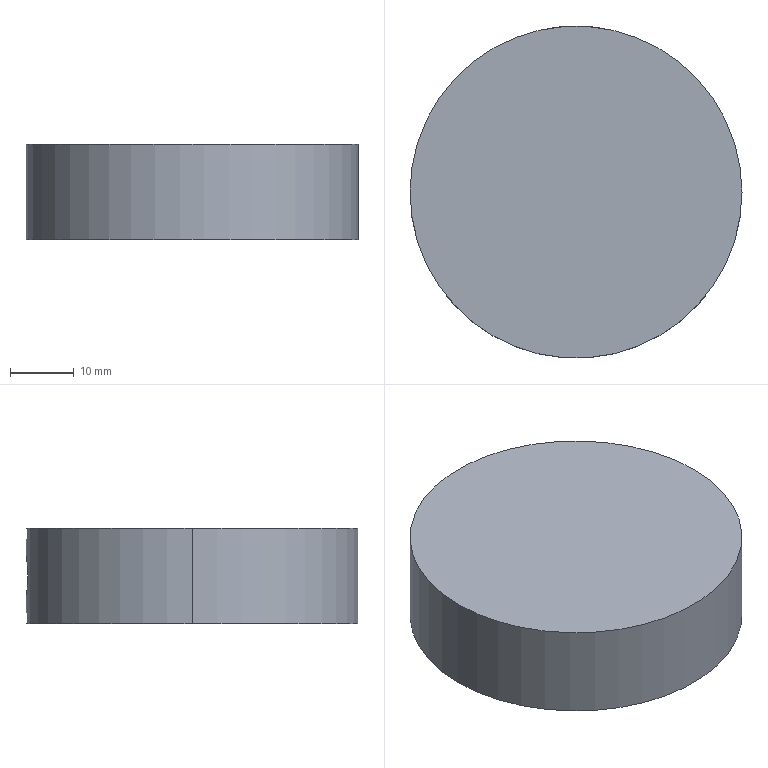Part | SolidWorks | features Extrusion 1, RevCut 1 | 1 solid | 8 faces | box 52 x 52 x 15 mm | volume 31469 mm3 | cylinder 4 | cone 2 | plane 2 | commonest cylinder face diameters 6.8 x2 52 x2
STEP:
#1=CARTESIAN_POINT('',(-106.5,85.3,0.));
#2=VERTEX_POINT('',#1);
#3=CARTESIAN_POINT('',(-109.9,87.263,0.));
#4=VERTEX_POINT('',#3);
#5=CARTESIAN_POINT('',(-106.5,85.3,0.));
#6=DIRECTION('',(-0.866,0.5,0.));
#7=VECTOR('',#6,1000.);
#8=LINE('',#5,#7);
#9=EDGE_CURVE('',#2,#4,#8,.T.);
#10=ORIENTED_EDGE('',*,*,#9,.F.);
#11=CARTESIAN_POINT('',(-103.1,87.263,0.));
#12=VERTEX_POINT('',#11);
#13=CARTESIAN_POINT('',(-106.5,85.3,0.));
#14=DIRECTION('',(0.866,0.5,0.));
#15=VECTOR('',#14,1000.);
#16=LINE('',#13,#15);
#17=EDGE_CURVE('',#2,#12,#16,.T.);
#18=ORIENTED_EDGE('',*,*,#17,.T.);
#19=CARTESIAN_POINT('',(-106.5,87.263,0.));
#20=DIRECTION('',(0.,-1.,0.));
#21=DIRECTION('',(1.,0.,0.));
#22=AXIS2_PLACEMENT_3D('',#19,#20,#21);
#23=CIRCLE('',#22,3.4);
#24=EDGE_CURVE('',#4,#12,#23,.T.);
#25=ORIENTED_EDGE('',*,*,#24,.F.);
#26=EDGE_LOOP('',(#10,#18,#25));
#27=FACE_OUTER_BOUND('',#26,.T.);
#28=CARTESIAN_POINT('',(-106.5,1085.3,0.));
#29=DIRECTION('',(0.,1.,0.));
#30=DIRECTION('',(-1.,0.,0.));
#31=AXIS2_PLACEMENT_3D('',#28,#29,#30);
#32=CONICAL_SURFACE('',#31,1732.051,1.047);
#33=ADVANCED_FACE('',(#27),#32,.F.);
#34=CARTESIAN_POINT('',(-109.9,97.077,0.));
#35=VERTEX_POINT('',#34);
#36=CARTESIAN_POINT('',(-103.1,97.077,0.));
#37=VERTEX_POINT('',#36);
#38=CARTESIAN_POINT('',(-109.9,97.077,0.));
#39=CARTESIAN_POINT('',(-109.9,97.077,-0.2248));
#40=CARTESIAN_POINT('',(-109.878,97.08,-0.4458));
#41=CARTESIAN_POINT('',(-109.791,97.091,-0.8807));
#42=CARTESIAN_POINT('',(-109.726,97.099,-1.097));
#43=CARTESIAN_POINT('',(-109.555,97.12,-1.508));
#44=CARTESIAN_POINT('',(-109.451,97.132,-1.703));
#45=CARTESIAN_POINT('',(-109.204,97.159,-2.073));
#46=CARTESIAN_POINT('',(-109.061,97.174,-2.248));
#47=CARTESIAN_POINT('',(-108.748,97.203,-2.561));
#48=CARTESIAN_POINT('',(-108.577,97.218,-2.701));
#49=CARTESIAN_POINT('',(-108.205,97.245,-2.95));
#50=CARTESIAN_POINT('',(-108.008,97.257,-3.056));
#51=CARTESIAN_POINT('',(-107.599,97.278,-3.225));
#52=CARTESIAN_POINT('',(-107.384,97.286,-3.291));
#53=CARTESIAN_POINT('',(-106.945,97.297,-3.378));
#54=CARTESIAN_POINT('',(-106.722,97.3,-3.4));
#55=CARTESIAN_POINT('',(-106.273,97.3,-3.4));
#56=CARTESIAN_POINT('',(-106.052,97.297,-3.378));
#57=CARTESIAN_POINT('',(-105.617,97.286,-3.291));
#58=CARTESIAN_POINT('',(-105.401,97.278,-3.225));
#59=CARTESIAN_POINT('',(-104.989,97.257,-3.054));
#60=CARTESIAN_POINT('',(-104.794,97.245,-2.95));
#61=CARTESIAN_POINT('',(-104.425,97.218,-2.703));
#62=CARTESIAN_POINT('',(-104.251,97.203,-2.559));
#63=CARTESIAN_POINT('',(-103.938,97.174,-2.246));
#64=CARTESIAN_POINT('',(-103.797,97.159,-2.075));
#65=CARTESIAN_POINT('',(-103.549,97.132,-1.703));
#66=CARTESIAN_POINT('',(-103.443,97.12,-1.505));
#67=CARTESIAN_POINT('',(-103.274,97.099,-1.096));
#68=CARTESIAN_POINT('',(-103.209,97.091,-0.8817));
#69=CARTESIAN_POINT('',(-103.122,97.08,-0.4427));
#70=CARTESIAN_POINT('',(-103.1,97.077,-0.222));
#71=CARTESIAN_POINT('',(-103.1,97.077,0.));
#72=B_SPLINE_CURVE_WITH_KNOTS('',3,(#38,#39,#40,#41,#42,#43,#44,#45,#46,#47,#48,#49,#50,#51,#52,#53,#54,#55,#56,#57,#58,#59,#60,#61,#62,#63,#64,#65,#66,#67,#68,#69,#70,#71),.UNSPECIFIED.,.F.,.F.,(4,2,2,2,2,2,2,2,2,2,2,2,2,2,2,2,4),(0.01596,0.01663,0.01729,0.01796,0.01862,0.01929,0.01995,0.02062,0.02128,0.02195,0.02261,0.02328,0.02394,0.02461,0.02527,0.02594,0.0266),.UNSPECIFIED.);
#73=EDGE_CURVE('',#35,#37,#72,.T.);
#74=ORIENTED_EDGE('',*,*,#73,.F.);
#75=CARTESIAN_POINT('',(-109.9,71.3,0.));
#76=DIRECTION('',(0.,-1.,0.));
#77=VECTOR('',#76,1000.);
#78=LINE('',#75,#77);
#79=EDGE_CURVE('',#35,#4,#78,.T.);
#80=ORIENTED_EDGE('',*,*,#79,.T.);
#81=ORIENTED_EDGE('',*,*,#24,.T.);
#82=CARTESIAN_POINT('',(-103.1,71.3,0.));
#83=DIRECTION('',(0.,-1.,0.));
#84=VECTOR('',#83,1000.);
#85=LINE('',#82,#84);
#86=EDGE_CURVE('',#37,#12,#85,.T.);
#87=ORIENTED_EDGE('',*,*,#86,.F.);
#88=EDGE_LOOP('',(#74,#80,#81,#87));
#89=FACE_OUTER_BOUND('',#88,.T.);
#90=CARTESIAN_POINT('',(-106.5,71.3,0.));
#91=DIRECTION('',(0.,-1.,0.));
#92=DIRECTION('',(1.,0.,0.));
#93=AXIS2_PLACEMENT_3D('',#90,#91,#92);
#94=CYLINDRICAL_SURFACE('',#93,3.4);
#95=ADVANCED_FACE('',(#89),#94,.F.);
#96=CARTESIAN_POINT('',(-103.1,97.077,0.));
#97=CARTESIAN_POINT('',(-103.1,97.077,0.222));
#98=CARTESIAN_POINT('',(-103.122,97.08,0.4476));
#99=CARTESIAN_POINT('',(-103.209,97.091,0.8838));
#100=CARTESIAN_POINT('',(-103.274,97.099,1.096));
#101=CARTESIAN_POINT('',(-103.444,97.12,1.508));
#102=CARTESIAN_POINT('',(-103.551,97.133,1.706));
#103=CARTESIAN_POINT('',(-103.797,97.159,2.074));
#104=CARTESIAN_POINT('',(-103.938,97.174,2.246));
#105=CARTESIAN_POINT('',(-104.255,97.203,2.563));
#106=CARTESIAN_POINT('',(-104.427,97.218,2.704));
#107=CARTESIAN_POINT('',(-104.795,97.245,2.95));
#108=CARTESIAN_POINT('',(-104.994,97.257,3.056));
#109=CARTESIAN_POINT('',(-105.405,97.278,3.227));
#110=CARTESIAN_POINT('',(-105.617,97.286,3.291));
#111=CARTESIAN_POINT('',(-106.054,97.297,3.378));
#112=CARTESIAN_POINT('',(-106.279,97.3,3.4));
#113=CARTESIAN_POINT('',(-106.723,97.3,3.4));
#114=CARTESIAN_POINT('',(-106.944,97.297,3.378));
#115=CARTESIAN_POINT('',(-107.383,97.286,3.291));
#116=CARTESIAN_POINT('',(-107.598,97.278,3.226));
#117=CARTESIAN_POINT('',(-108.007,97.257,3.056));
#118=CARTESIAN_POINT('',(-108.205,97.245,2.95));
#119=CARTESIAN_POINT('',(-108.576,97.218,2.702));
#120=CARTESIAN_POINT('',(-108.747,97.203,2.561));
#121=CARTESIAN_POINT('',(-109.061,97.174,2.248));
#122=CARTESIAN_POINT('',(-109.204,97.159,2.073));
#123=CARTESIAN_POINT('',(-109.451,97.132,1.704));
#124=CARTESIAN_POINT('',(-109.555,97.12,1.509));
#125=CARTESIAN_POINT('',(-109.726,97.099,1.097));
#126=CARTESIAN_POINT('',(-109.791,97.091,0.8809));
#127=CARTESIAN_POINT('',(-109.878,97.08,0.4461));
#128=CARTESIAN_POINT('',(-109.9,97.077,0.2248));
#129=CARTESIAN_POINT('',(-109.9,97.077,0.));
#130=B_SPLINE_CURVE_WITH_KNOTS('',3,(#96,#97,#98,#99,#100,#101,#102,#103,#104,#105,#106,#107,#108,#109,#110,#111,#112,#113,#114,#115,#116,#117,#118,#119,#120,#121,#122,#123,#124,#125,#126,#127,#128,#129),.UNSPECIFIED.,.F.,.F.,(4,2,2,2,2,2,2,2,2,2,2,2,2,2,2,2,4),(0.005322,0.005987,0.006652,0.007317,0.007982,0.008647,0.009312,0.009977,0.01064,0.01131,0.01197,0.01264,0.0133,0.01397,0.01463,0.0153,0.01596),.UNSPECIFIED.);
#131=EDGE_CURVE('',#37,#35,#130,.T.);
#132=ORIENTED_EDGE('',*,*,#131,.T.);
#133=ORIENTED_EDGE('',*,*,#73,.T.);
#134=EDGE_LOOP('',(#132,#133));
#135=FACE_BOUND('',#134,.T.);
#136=CARTESIAN_POINT('',(-80.5,71.3,7.5));
#137=VERTEX_POINT('',#136);
#138=CARTESIAN_POINT('',(-132.5,71.3,7.5));
#139=VERTEX_POINT('',#138);
#140=CARTESIAN_POINT('',(-106.5,71.3,7.5));
#141=DIRECTION('',(0.,0.,1.));
#142=DIRECTION('',(1.,0.,0.));
#143=AXIS2_PLACEMENT_3D('',#140,#141,#142);
#144=CIRCLE('',#143,26.);
#145=EDGE_CURVE('',#137,#139,#144,.T.);
#146=ORIENTED_EDGE('',*,*,#145,.F.);
#147=CARTESIAN_POINT('',(-80.5,71.3,-7.5));
#148=VERTEX_POINT('',#147);
#149=CARTESIAN_POINT('',(-80.5,71.3,7.5));
#150=DIRECTION('',(0.,0.,-1.));
#151=VECTOR('',#150,1000.);
#152=LINE('',#149,#151);
#153=EDGE_CURVE('',#137,#148,#152,.T.);
#154=ORIENTED_EDGE('',*,*,#153,.T.);
#155=CARTESIAN_POINT('',(-132.5,71.3,-7.5));
#156=VERTEX_POINT('',#155);
#157=CARTESIAN_POINT('',(-106.5,71.3,-7.5));
#158=DIRECTION('',(0.,0.,1.));
#159=DIRECTION('',(1.,0.,0.));
#160=AXIS2_PLACEMENT_3D('',#157,#158,#159);
#161=CIRCLE('',#160,26.);
#162=EDGE_CURVE('',#148,#156,#161,.T.);
#163=ORIENTED_EDGE('',*,*,#162,.T.);
#164=CARTESIAN_POINT('',(-132.5,71.3,7.5));
#165=DIRECTION('',(0.,0.,-1.));
#166=VECTOR('',#165,1000.);
#167=LINE('',#164,#166);
#168=EDGE_CURVE('',#139,#156,#167,.T.);
#169=ORIENTED_EDGE('',*,*,#168,.F.);
#170=EDGE_LOOP('',(#146,#154,#163,#169));
#171=FACE_OUTER_BOUND('',#170,.T.);
#172=CARTESIAN_POINT('',(-106.5,71.3,7.5));
#173=DIRECTION('',(0.,0.,-1.));
#174=DIRECTION('',(-1.,0.,0.));
#175=AXIS2_PLACEMENT_3D('',#172,#173,#174);
#176=CYLINDRICAL_SURFACE('',#175,26.);
#177=ADVANCED_FACE('',(#135,#171),#176,.T.);
#178=ORIENTED_EDGE('',*,*,#153,.F.);
#179=CARTESIAN_POINT('',(-106.5,71.3,7.5));
#180=DIRECTION('',(0.,0.,1.));
#181=DIRECTION('',(1.,0.,0.));
#182=AXIS2_PLACEMENT_3D('',#179,#180,#181);
#183=CIRCLE('',#182,26.);
#184=EDGE_CURVE('',#139,#137,#183,.T.);
#185=ORIENTED_EDGE('',*,*,#184,.F.);
#186=ORIENTED_EDGE('',*,*,#168,.T.);
#187=CARTESIAN_POINT('',(-106.5,71.3,-7.5));
#188=DIRECTION('',(0.,0.,1.));
#189=DIRECTION('',(1.,0.,0.));
#190=AXIS2_PLACEMENT_3D('',#187,#188,#189);
#191=CIRCLE('',#190,26.);
#192=EDGE_CURVE('',#156,#148,#191,.T.);
#193=ORIENTED_EDGE('',*,*,#192,.T.);
#194=EDGE_LOOP('',(#178,#185,#186,#193));
#195=FACE_OUTER_BOUND('',#194,.T.);
#196=CARTESIAN_POINT('',(-106.5,71.3,7.5));
#197=DIRECTION('',(0.,0.,-1.));
#198=DIRECTION('',(-1.,0.,0.));
#199=AXIS2_PLACEMENT_3D('',#196,#197,#198);
#200=CYLINDRICAL_SURFACE('',#199,26.);
#201=ADVANCED_FACE('',(#195),#200,.T.);
#202=ORIENTED_EDGE('',*,*,#184,.T.);
#203=ORIENTED_EDGE('',*,*,#145,.T.);
#204=EDGE_LOOP('',(#202,#203));
#205=FACE_OUTER_BOUND('',#204,.T.);
#206=CARTESIAN_POINT('',(-106.5,71.3,7.5));
#207=DIRECTION('',(0.,0.,1.));
#208=DIRECTION('',(1.,0.,0.));
#209=AXIS2_PLACEMENT_3D('',#206,#207,#208);
#210=PLANE('',#209);
#211=ADVANCED_FACE('',(#205),#210,.T.);
#212=ORIENTED_EDGE('',*,*,#192,.F.);
#213=ORIENTED_EDGE('',*,*,#162,.F.);
#214=EDGE_LOOP('',(#212,#213));
#215=FACE_OUTER_BOUND('',#214,.T.);
#216=CARTESIAN_POINT('',(-106.5,71.3,-7.5));
#217=DIRECTION('',(0.,0.,1.));
#218=DIRECTION('',(1.,0.,0.));
#219=AXIS2_PLACEMENT_3D('',#216,#217,#218);
#220=PLANE('',#219);
#221=ADVANCED_FACE('',(#215),#220,.F.);
#222=ORIENTED_EDGE('',*,*,#79,.F.);
#223=ORIENTED_EDGE('',*,*,#131,.F.);
#224=ORIENTED_EDGE('',*,*,#86,.T.);
#225=CARTESIAN_POINT('',(-106.5,87.263,0.));
#226=DIRECTION('',(0.,-1.,0.));
#227=DIRECTION('',(1.,0.,0.));
#228=AXIS2_PLACEMENT_3D('',#225,#226,#227);
#229=CIRCLE('',#228,3.4);
#230=EDGE_CURVE('',#12,#4,#229,.T.);
#231=ORIENTED_EDGE('',*,*,#230,.T.);
#232=EDGE_LOOP('',(#222,#223,#224,#231));
#233=FACE_OUTER_BOUND('',#232,.T.);
#234=CARTESIAN_POINT('',(-106.5,71.3,0.));
#235=DIRECTION('',(0.,-1.,0.));
#236=DIRECTION('',(1.,0.,0.));
#237=AXIS2_PLACEMENT_3D('',#234,#235,#236);
#238=CYLINDRICAL_SURFACE('',#237,3.4);
#239=ADVANCED_FACE('',(#233),#238,.F.);
#240=ORIENTED_EDGE('',*,*,#17,.F.);
#241=ORIENTED_EDGE('',*,*,#9,.T.);
#242=ORIENTED_EDGE('',*,*,#230,.F.);
#243=EDGE_LOOP('',(#240,#241,#242));
#244=FACE_OUTER_BOUND('',#243,.T.);
#245=CARTESIAN_POINT('',(-106.5,1085.3,0.));
#246=DIRECTION('',(0.,1.,0.));
#247=DIRECTION('',(-1.,0.,0.));
#248=AXIS2_PLACEMENT_3D('',#245,#246,#247);
#249=CONICAL_SURFACE('',#248,1732.051,1.047);
#250=ADVANCED_FACE('',(#244),#249,.F.);
#251=CLOSED_SHELL('',(#33,#95,#177,#201,#211,#221,#239,#250));
#252=MANIFOLD_SOLID_BREP('',#251);
#253=CARTESIAN_POINT('',(0.,0.,0.));
#254=DIRECTION('',(0.,0.,1.));
#255=DIRECTION('',(1.,0.,0.));
#256=AXIS2_PLACEMENT_3D('',#253,#254,#255);
#257=(LENGTH_UNIT()NAMED_UNIT(*)SI_UNIT(.MILLI.,.METRE.));
#258=UNCERTAINTY_MEASURE_WITH_UNIT(LENGTH_MEASURE(0.00001),#257,'','');
#259=(NAMED_UNIT(*)PLANE_ANGLE_UNIT()SI_UNIT($,.RADIAN.));
#260=(NAMED_UNIT(*)SI_UNIT($,.STERADIAN.)SOLID_ANGLE_UNIT());
#261=(GEOMETRIC_REPRESENTATION_CONTEXT(3)GLOBAL_UNCERTAINTY_ASSIGNED_CONTEXT((#258))GLOBAL_UNIT_ASSIGNED_CONTEXT((#257,#259,#260))REPRESENTATION_CONTEXT('',''));
#262=ADVANCED_BREP_SHAPE_REPRESENTATION('',(#252,#256),#261);